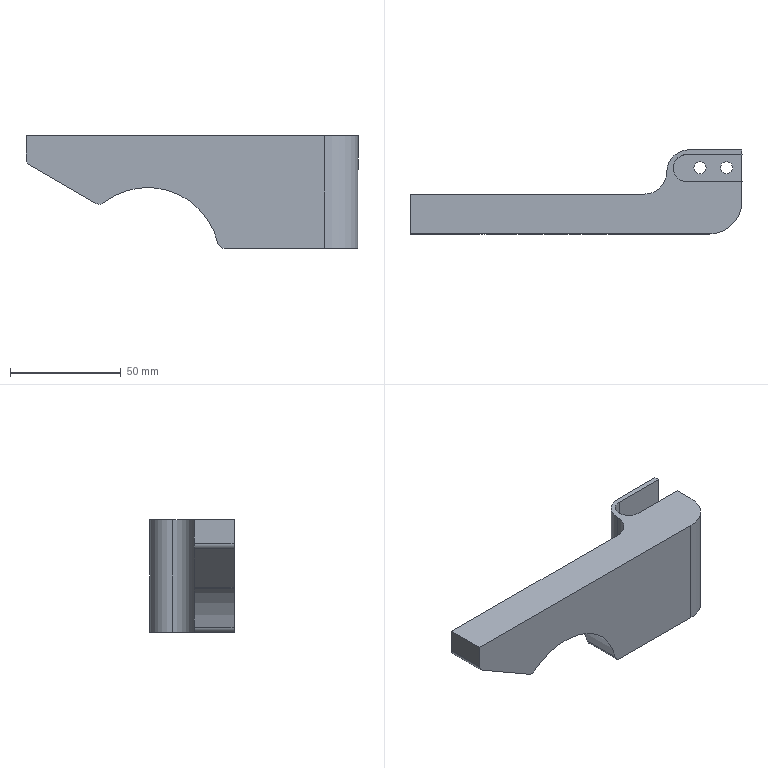NC program | NX | posted with a generic post | part box 150 x 38 x 51 mm
Lines 4811 to 5633 of 31037:
(FIXED_CONTOUR , TOOL : R4)
N9572 T08 M6
N9574 G54
N9576 G17 G0 G90 X11.552 Y21.893 S9500 M3
N9578 G43 Z30. H8
N9580 Z3.895
N9582 G94 G1 X11.585 Y21.86 Z3.374 F3000.
N9584 X11.666 Y21.779 Z2.863
N9586 X11.793 Y21.652 Z2.372
N9588 X11.964 Y21.481 Z1.908
N9590 X12.177 Y21.268 Z1.48
N9592 X12.427 Y21.018 Z1.095
N9594 X12.711 Y20.734 Z0.759
N9596 X13.023 Y20.421 Z0.479
N9598 X13.359 Y20.086 Z0.258
N9600 X13.712 Y19.733 Z0.102
N9602 X14.077 Y19.368 Z0.012
N9604 X14.446 Y18.999 Z-0.01
N9606 X14.583 Y18.862 Z-0.005
N9608 Y18.725 Z-0.004
N9610 X14.309 Y18.999 Z-0.013
N9612 X14.173 Z-0.016
N9614 X14.583 Y18.589 Z-0.003
N9616 Y18.452
N9618 X14.16 Y18.876 Z-0.016
N9620 X14.036 Y19. Z-0.027
N9622 X13.899 Z-0.039
N9624 X14.16 Y18.739 Z-0.014
N9626 X14.583 Y18.316 Z-0.003
N9628 Y18.18
N9630 X14.16 Y18.603 Z-0.013
N9632 X13.877 Y18.886 Z-0.04
N9634 X13.763 Y19. Z-0.054
N9636 X13.626 Z-0.07
N9638 X13.877 Y18.749 Z-0.038
N9640 X14.16 Y18.467 Z-0.013
N9642 X14.583 Y18.043 Z-0.003
N9644 Y17.907
N9646 X14.16 Y18.331 Z-0.013
N9648 X13.84 Y18.65 Z-0.042
N9650 X13.594 Y18.896 Z-0.073
N9652 X13.491 Y19. Z-0.092
N9654 X13.356 Z-0.115
N9656 X13.594 Y18.762 Z-0.071
N9658 X13.877 Y18.479 Z-0.037
N9660 X14.16 Y18.196 Z-0.013
N9662 X14.583 Y17.773 Z-0.003
N9664 Y17.638
N9666 X14.16 Y18.061 Z-0.013
N9668 X13.877 Y18.344 Z-0.037
N9670 X13.594 Y18.626 Z-0.07
N9672 X13.311 Y18.909 Z-0.122
N9674 X13.221 Y19. Z-0.143
N9676 X13.085 Z-0.174
N9678 X13.311 Y18.774 Z-0.121
N9680 X13.594 Y18.491 Z-0.07
N9682 X13.877 Y18.208 Z-0.037
N9684 X14.16 Y17.926 Z-0.013
N9686 X14.583 Y17.502 Z-0.003
N9688 Y17.367
N9690 X14.16 Y17.791 Z-0.013
N9692 X13.877 Y18.073 Z-0.037
N9694 X13.594 Y18.356 Z-0.07
N9696 X13.3 Y18.65 Z-0.122
N9698 X12.95 Y19. Z-0.205
N9700 X12.816 Z-0.236
N9702 X13.165 Y18.65 Z-0.152
N9704 X13.311 Y18.504 Z-0.119
N9706 X13.594 Y18.222 Z-0.07
N9708 X13.877 Y17.939 Z-0.037
N9710 X14.16 Y17.656 Z-0.013
N9712 X14.583 Y17.233 Z-0.003
N9714 Y17.1
N9716 X14.16 Y17.523 Z-0.013
N9718 X13.877 Y17.806 Z-0.037
N9720 X13.594 Y18.088 Z-0.07
N9722 X13.311 Y18.371 Z-0.119
N9724 X13.032 Y18.65 Z-0.182
N9726 X12.746 Y18.937 Z-0.251
N9728 X12.683 Y19. Z-0.27
N9730 X12.549 Z-0.308
N9732 X12.746 Y18.803 Z-0.25
N9734 X13.029 Y18.52 Z-0.183
N9736 X13.311 Y18.237 Z-0.119
N9738 X13.594 Y17.955 Z-0.07
N9740 X13.877 Y17.672 Z-0.037
N9742 X14.16 Y17.389 Z-0.013
N9744 X14.583 Y16.966 Z-0.003
N9746 Y16.832
N9748 X14.16 Y17.256 Z-0.013
N9750 X13.878 Y17.537 Z-0.037
N9752 X13.594 Y17.821 Z-0.07
N9754 X13.311 Y18.104 Z-0.119
N9756 X12.746 Y18.669 Z-0.248
N9758 X12.463 Y18.952 Z-0.332
N9760 X12.415 Y19. Z-0.35
N9762 X12.284 Z-0.398
N9764 X12.463 Y18.821 Z-0.331
N9766 X12.746 Y18.538 Z-0.248
N9768 X13.311 Y17.973 Z-0.119
N9770 X13.594 Y17.69 Z-0.07
N9772 X13.877 Y17.407 Z-0.037
N9774 X14.16 Y17.124 Z-0.013
N9776 X14.583 Y16.701 Z-0.003
N9778 Y16.569
N9780 X14.16 Y16.993 Z-0.013
N9782 X13.877 Y17.275 Z-0.037
N9784 X13.594 Y17.558 Z-0.07
N9786 X13.311 Y17.841 Z-0.119
N9788 X12.746 Y18.406 Z-0.248
N9790 X12.463 Y18.689 Z-0.329
N9792 X12.152 Y19. Z-0.447
N9794 X12.02 Z-0.499
N9796 X12.181 Y18.84 Z-0.434
N9798 X12.463 Y18.557 Z-0.329
N9800 X12.746 Y18.274 Z-0.248
N9802 X13.311 Y17.709 Z-0.119
N9804 X13.594 Y17.426 Z-0.07
N9806 X13.877 Y17.143 Z-0.037
N9808 X14.16 Y16.861 Z-0.013
N9810 X14.583 Y16.437 Z-0.003
N9812 Y16.305
N9814 X14.16 Y16.728 Z-0.013
N9816 X13.877 Y17.011 Z-0.037
N9818 X13.594 Y17.294 Z-0.07
N9820 X13.311 Y17.577 Z-0.119
N9822 X12.746 Y18.142 Z-0.248
N9824 X12.463 Y18.425 Z-0.329
N9826 X12.181 Y18.708 Z-0.433
N9828 X11.888 Y19. Z-0.551
N9830 X11.757 Z-0.605
N9832 X11.898 Y18.859 Z-0.545
N9834 X12.181 Y18.576 Z-0.432
N9836 X12.463 Y18.294 Z-0.329
N9838 X12.746 Y18.011 Z-0.248
N9840 X13.311 Y17.445 Z-0.119
N9842 X13.594 Y17.163 Z-0.07
N9844 X13.877 Y16.88 Z-0.037
N9846 X14.16 Y16.597 Z-0.013
N9848 X14.583 Y16.174 Z-0.003
N9850 Y16.044
N9852 X14.16 Y16.467 Z-0.013
N9854 X13.877 Y16.75 Z-0.037
N9856 X13.594 Y17.032 Z-0.07
N9858 X13.311 Y17.315 Z-0.119
N9860 X12.746 Y17.881 Z-0.248
N9862 X12.463 Y18.163 Z-0.329
N9864 X12.181 Y18.446 Z-0.432
N9866 X11.898 Y18.729 Z-0.544
N9868 X11.626 Y19. Z-0.66
N9870 X11.502 Z-0.722
N9872 X11.615 Y18.887 Z-0.663
N9874 X11.898 Y18.604 Z-0.543
N9876 X12.181 Y18.321 Z-0.432
N9878 X12.463 Y18.039 Z-0.329
N9880 X12.746 Y17.756 Z-0.248
N9882 X13.311 Y17.19 Z-0.119
N9884 X13.594 Y16.908 Z-0.07
N9886 X13.877 Y16.625 Z-0.037
N9888 X14.16 Y16.342 Z-0.013
N9890 X14.583 Y15.919 Z-0.003
N9892 Y15.79
N9894 X14.16 Y16.214 Z-0.013
N9896 X13.877 Y16.496 Z-0.037
N9898 X13.594 Y16.779 Z-0.07
N9900 X13.311 Y17.062 Z-0.119
N9902 X12.746 Y17.627 Z-0.248
N9904 X12.463 Y17.91 Z-0.329
N9906 X12.181 Y18.193 Z-0.432
N9908 X11.898 Y18.475 Z-0.543
N9910 X11.615 Y18.758 Z-0.662
N9912 X11.373 Y19. Z-0.787
N9914 X11.332 Z-0.808
N9916 X11.245 Z-0.858
N9918 X11.332 Y18.913 Z-0.807
N9920 X11.615 Y18.63 Z-0.661
N9922 X11.898 Y18.347 Z-0.543
N9924 X12.181 Y18.065 Z-0.432
N9926 X12.463 Y17.782 Z-0.329
N9928 X12.746 Y17.499 Z-0.248
N9930 X13.311 Y16.934 Z-0.119
N9932 X13.594 Y16.651 Z-0.07
N9934 X13.877 Y16.368 Z-0.037
N9936 X14.16 Y16.085 Z-0.013
N9938 X14.583 Y15.662 Z-0.003
N9940 Y15.536
N9942 X14.16 Y15.959 Z-0.013
N9944 X13.877 Y16.242 Z-0.037
N9946 X13.594 Y16.524 Z-0.07
N9948 X13.311 Y16.807 Z-0.119
N9950 X12.746 Y17.373 Z-0.248
N9952 X12.463 Y17.655 Z-0.329
N9954 X12.181 Y17.938 Z-0.432
N9956 X11.898 Y18.221 Z-0.543
N9958 X11.615 Y18.504 Z-0.661
N9960 X11.332 Y18.786 Z-0.806
N9962 X11.119 Y19. Z-0.931
N9964 X10.994 Z-1.003
N9966 X11.344 Y18.65 Z-0.798
N9968 X11.615 Y18.379 Z-0.661
N9970 X11.902 Y18.092 Z-0.541
N9972 X12.181 Y17.814 Z-0.432
N9974 X12.463 Y17.531 Z-0.329
N9976 X12.746 Y17.248 Z-0.248
N9978 X13.311 Y16.683 Z-0.119
N9980 X13.594 Y16.4 Z-0.07
N9982 X13.877 Y16.117 Z-0.037
N9984 X14.16 Y15.835 Z-0.013
N9986 X14.583 Y15.411 Z-0.003
N9988 Y15.286
N9990 X14.16 Y15.709 Z-0.013
N9992 X13.877 Y15.992 Z-0.037
N9994 X13.594 Y16.275 Z-0.07
N9996 X13.311 Y16.558 Z-0.119
N9998 X12.746 Y17.123 Z-0.248
N10000 X12.463 Y17.406 Z-0.329
N10002 X12.181 Y17.689 Z-0.432
N10004 X11.898 Y17.971 Z-0.543
N10006 X11.615 Y18.254 Z-0.661
N10008 X11.332 Y18.537 Z-0.804
N10010 X11.05 Y18.819 Z-0.969
N10012 X10.869 Y19. Z-1.077
N10014 X10.767 Z-1.137
N10016 X10.743 Z-1.153
N10018 X10.767 Y18.976 Z-1.137
N10020 X11.093 Y18.65 Z-0.942
N10022 X11.332 Y18.411 Z-0.804
N10024 X11.615 Y18.128 Z-0.661
N10026 X11.898 Y17.846 Z-0.543
N10028 X12.181 Y17.563 Z-0.432
N10030 X12.463 Y17.28 Z-0.329
N10032 X12.746 Y16.997 Z-0.248
N10034 X13.311 Y16.432 Z-0.119
N10036 X13.594 Y16.149 Z-0.07
N10038 X13.879 Y15.864 Z-0.037
N10040 X14.16 Y15.584 Z-0.013
N10042 X14.583 Y15.16 Z-0.003
N10044 Y15.039
N10046 X14.16 Y15.462 Z-0.013
N10048 X13.877 Y15.745 Z-0.037
N10050 X13.594 Y16.027 Z-0.07
N10052 X13.311 Y16.31 Z-0.119
N10054 X12.746 Y16.876 Z-0.248
N10056 X12.463 Y17.158 Z-0.329
N10058 X12.181 Y17.441 Z-0.432
N10060 X11.898 Y17.724 Z-0.543
N10062 X11.615 Y18.007 Z-0.661
N10064 X11.332 Y18.289 Z-0.804
N10066 X10.971 Y18.65 Z-1.013
N10068 X10.767 Y18.855 Z-1.135
N10070 X10.622 Y19. Z-1.237
N10072 X10.499 Z-1.322
N10074 X10.767 Y18.733 Z-1.134
N10076 X11.05 Y18.45 Z-0.967
N10078 X11.332 Y18.167 Z-0.804
N10080 X11.615 Y17.884 Z-0.661
N10082 X11.898 Y17.602 Z-0.543
N10084 X12.181 Y17.319 Z-0.432
N10086 X12.463 Y17.036 Z-0.329
N10088 X12.746 Y16.754 Z-0.248
N10090 X13.311 Y16.188 Z-0.119
N10092 X13.594 Y15.905 Z-0.07
N10094 X13.877 Y15.623 Z-0.037
N10096 X14.16 Y15.34 Z-0.013
N10098 X14.583 Y14.917 Z-0.003
N10100 Y14.795
N10102 X14.16 Y15.219 Z-0.013
N10104 X13.877 Y15.501 Z-0.037
N10106 X13.594 Y15.784 Z-0.07
N10108 X13.311 Y16.067 Z-0.119
N10110 X12.746 Y16.632 Z-0.248
N10112 X12.463 Y16.915 Z-0.329
N10114 X12.181 Y17.198 Z-0.432
N10116 X11.898 Y17.481 Z-0.543
N10118 X11.615 Y17.763 Z-0.661
N10120 X11.332 Y18.046 Z-0.804
N10122 X11.05 Y18.329 Z-0.967
N10124 X10.767 Y18.611 Z-1.133
N10126 X10.484 Y18.894 Z-1.331
N10128 X10.378 Y19. Z-1.416
N10130 X10.259 Z-1.511
N10132 X10.484 Y18.775 Z-1.33
N10134 X10.767 Y18.492 Z-1.133
N10136 X11.05 Y18.209 Z-0.967
N10138 X11.332 Y17.926 Z-0.804
N10140 X11.615 Y17.644 Z-0.661
N10142 X11.898 Y17.361 Z-0.543
N10144 X12.181 Y17.078 Z-0.432
N10146 X12.463 Y16.795 Z-0.329
N10148 X12.746 Y16.513 Z-0.248
N10150 X13.311 Y15.947 Z-0.119
N10152 X13.594 Y15.664 Z-0.07
N10154 X13.877 Y15.382 Z-0.037
N10156 X14.16 Y15.099 Z-0.013
N10158 X14.583 Y14.676 Z-0.003
N10160 Y14.558
N10162 X14.16 Y14.982 Z-0.013
N10164 X13.877 Y15.264 Z-0.037
N10166 X13.594 Y15.547 Z-0.07
N10168 X13.311 Y15.83 Z-0.119
N10170 X12.746 Y16.395 Z-0.248
N10172 X12.463 Y16.678 Z-0.329
N10174 X12.181 Y16.961 Z-0.432
N10176 X11.898 Y17.243 Z-0.543
N10178 X11.615 Y17.526 Z-0.661
N10180 X11.332 Y17.809 Z-0.804
N10182 X11.05 Y18.092 Z-0.967
N10184 X10.767 Y18.374 Z-1.133
N10186 X10.484 Y18.657 Z-1.328
N10188 X10.141 Y19. Z-1.605
N10190 X10.027 Z-1.698
N10192 X10.201 Y18.826 Z-1.554
N10194 X10.484 Y18.543 Z-1.328
N10196 X10.767 Y18.26 Z-1.133
N10198 X11.05 Y17.977 Z-0.967
N10200 X11.332 Y17.695 Z-0.804
N10202 X11.615 Y17.412 Z-0.661
N10204 X11.898 Y17.129 Z-0.543
N10206 X12.181 Y16.847 Z-0.432
N10208 X12.463 Y16.564 Z-0.329
N10210 X12.746 Y16.281 Z-0.248
N10212 X13.311 Y15.716 Z-0.119
N10214 X13.594 Y15.433 Z-0.07
N10216 X13.877 Y15.15 Z-0.037
N10218 X14.16 Y14.867 Z-0.013
N10220 X14.583 Y14.444 Z-0.003
N10222 Y14.326
N10224 X14.16 Y14.75 Z-0.013
N10226 X13.877 Y15.033 Z-0.037
N10228 X13.594 Y15.315 Z-0.07
N10230 X13.311 Y15.598 Z-0.119
N10232 X12.746 Y16.163 Z-0.248
N10234 X12.463 Y16.446 Z-0.329
N10236 X12.181 Y16.729 Z-0.432
N10238 X11.898 Y17.012 Z-0.543
N10240 X11.615 Y17.294 Z-0.661
N10242 X11.332 Y17.577 Z-0.804
N10244 X11.05 Y17.86 Z-0.967
N10246 X10.767 Y18.143 Z-1.133
N10248 X10.484 Y18.425 Z-1.328
N10250 X10.201 Y18.708 Z-1.552
N10252 X9.909 Y19. Z-1.795
N10254 X9.798 Z-1.902
N10256 X9.919 Y18.879 Z-1.784
N10258 X10.201 Y18.597 Z-1.551
N10260 X10.484 Y18.314 Z-1.328
N10262 X10.767 Y18.031 Z-1.133
N10264 X11.05 Y17.748 Z-0.967
N10266 X11.332 Y17.466 Z-0.804
N10268 X11.615 Y17.183 Z-0.661
N10270 X11.898 Y16.9 Z-0.543
N10272 X12.181 Y16.617 Z-0.432
N10274 X12.463 Y16.335 Z-0.329
N10276 X12.746 Y16.052 Z-0.248
N10278 X13.311 Y15.486 Z-0.119
N10280 X13.594 Y15.204 Z-0.07
N10282 X13.877 Y14.921 Z-0.037
N10284 X14.16 Y14.638 Z-0.013
N10286 X14.583 Y14.215 Z-0.003
N10288 Y14.102
N10290 X14.16 Y14.525 Z-0.013
N10292 X13.877 Y14.808 Z-0.037
N10294 X13.594 Y15.091 Z-0.07
N10296 X13.311 Y15.374 Z-0.119
N10298 X12.746 Y15.939 Z-0.248
N10300 X12.463 Y16.222 Z-0.329
N10302 X12.181 Y16.505 Z-0.432
N10304 X11.898 Y16.787 Z-0.543
N10306 X11.615 Y17.07 Z-0.661
N10308 X11.332 Y17.353 Z-0.804
N10310 X11.05 Y17.636 Z-0.967
N10312 X10.767 Y17.918 Z-1.133
N10314 X10.484 Y18.201 Z-1.328
N10316 X10.201 Y18.484 Z-1.551
N10318 X9.919 Y18.766 Z-1.783
N10320 X9.685 Y19. Z-2.01
N10322 X9.636 Z-2.056
N10324 X9.572 Z-2.124
N10326 X9.636 Y18.936 Z-2.054
N10328 X9.919 Y18.654 Z-1.781
N10330 X10.201 Y18.371 Z-1.551
N10332 X10.484 Y18.088 Z-1.328
N10334 X10.767 Y17.806 Z-1.133
N10336 X11.05 Y17.523 Z-0.967
N10338 X11.332 Y17.24 Z-0.804
N10340 X11.615 Y16.957 Z-0.661
N10342 X11.898 Y16.675 Z-0.543
N10344 X12.181 Y16.392 Z-0.432
N10346 X12.463 Y16.109 Z-0.329
N10348 X12.746 Y15.826 Z-0.248
N10350 X13.311 Y15.261 Z-0.119
N10352 X13.594 Y14.978 Z-0.07
N10354 X13.877 Y14.695 Z-0.037
N10356 X14.16 Y14.413 Z-0.013
N10358 X14.583 Y13.989 Z-0.003
N10360 Y13.88
N10362 X14.16 Y14.303 Z-0.013
N10364 X13.877 Y14.586 Z-0.037
N10366 X13.594 Y14.869 Z-0.07
N10368 X13.311 Y15.151 Z-0.119
N10370 X12.746 Y15.717 Z-0.248
N10372 X12.463 Y16. Z-0.329
N10374 X12.181 Y16.282 Z-0.432
N10376 X11.898 Y16.565 Z-0.543
N10378 X11.615 Y16.848 Z-0.661
N10380 X11.332 Y17.131 Z-0.804
N10382 X11.05 Y17.413 Z-0.967
N10384 X10.767 Y17.696 Z-1.133
N10386 X10.484 Y17.979 Z-1.328
N10388 X10.201 Y18.262 Z-1.551
N10390 X9.919 Y18.544 Z-1.781
N10392 X9.636 Y18.827 Z-2.053
N10394 X9.463 Y19. Z-2.241
N10396 X9.357 Z-2.355
N10398 X9.636 Y18.721 Z-2.053
N10400 X9.919 Y18.438 Z-1.781
N10402 X10.201 Y18.156 Z-1.551
N10404 X10.484 Y17.873 Z-1.328
N10406 X10.767 Y17.59 Z-1.133
N10408 X11.05 Y17.307 Z-0.967
N10410 X11.332 Y17.025 Z-0.804
N10412 X11.615 Y16.742 Z-0.661
N10414 X11.898 Y16.459 Z-0.543
N10416 X12.181 Y16.176 Z-0.432
N10418 X12.463 Y15.894 Z-0.329
N10420 X12.746 Y15.611 Z-0.248
N10422 X13.311 Y15.045 Z-0.119
N10424 X13.594 Y14.763 Z-0.07
N10426 X13.877 Y14.48 Z-0.037
N10428 X14.16 Y14.197 Z-0.013
N10430 X14.583 Y13.774 Z-0.003
N10432 Y13.669
N10434 X14.16 Y14.092 Z-0.013
N10436 X13.877 Y14.375 Z-0.037
N10438 X13.594 Y14.657 Z-0.07
N10440 X13.311 Y14.94 Z-0.119
N10442 X12.746 Y15.506 Z-0.248
N10444 X12.463 Y15.788 Z-0.329
N10446 X12.181 Y16.071 Z-0.432
N10448 X11.898 Y16.354 Z-0.543
N10450 X11.615 Y16.637 Z-0.661
N10452 X11.332 Y16.919 Z-0.804
N10454 X11.05 Y17.202 Z-0.967
N10456 X10.767 Y17.485 Z-1.133
N10458 X10.484 Y17.768 Z-1.328
N10460 X10.201 Y18.05 Z-1.551
N10462 X9.919 Y18.333 Z-1.781
N10464 X9.636 Y18.616 Z-2.053
N10466 X9.353 Y18.898 Z-2.357
N10468 X9.252 Y19. Z-2.477
N10470 X9.147 Z-2.599
N10472 X9.353 Y18.794 Z-2.357
N10474 X9.636 Y18.511 Z-2.053
N10476 X9.919 Y18.229 Z-1.781
N10478 X10.201 Y17.946 Z-1.551
N10480 X10.484 Y17.663 Z-1.328
N10482 X10.767 Y17.381 Z-1.133
N10484 X11.05 Y17.098 Z-0.967
N10486 X11.332 Y16.815 Z-0.804
N10488 X11.615 Y16.532 Z-0.661
N10490 X11.898 Y16.25 Z-0.543
N10492 X12.181 Y15.967 Z-0.432
N10494 X12.463 Y15.684 Z-0.329
N10496 X12.746 Y15.401 Z-0.248
N10498 X13.311 Y14.836 Z-0.119
N10500 X13.594 Y14.553 Z-0.07
N10502 X13.877 Y14.27 Z-0.037
N10504 X14.16 Y13.988 Z-0.013
N10506 X14.583 Y13.564 Z-0.003
N10508 Y13.464
N10510 X14.16 Y13.887 Z-0.013
N10512 X13.877 Y14.17 Z-0.037
N10514 X13.594 Y14.453 Z-0.07
N10516 X13.311 Y14.736 Z-0.119
N10518 X12.746 Y15.301 Z-0.248
N10520 X12.463 Y15.584 Z-0.329
N10522 X12.183 Y15.864 Z-0.431
N10524 X11.898 Y16.149 Z-0.543
N10526 X11.615 Y16.432 Z-0.661
N10528 X11.332 Y16.715 Z-0.804
N10530 X11.057 Y16.99 Z-0.963
N10532 X10.767 Y17.28 Z-1.133
N10534 X10.484 Y17.563 Z-1.328
N10536 X10.201 Y17.846 Z-1.551
N10538 X9.919 Y18.128 Z-1.781
N10540 X9.636 Y18.411 Z-2.053
N10542 X9.353 Y18.694 Z-2.357
N10544 X9.07 Y18.977 Z-2.687
N10546 X9.047 Y19. Z-2.722
N10548 X8.951 Z-2.858
N10550 X9.07 Y18.881 Z-2.686
N10552 X9.353 Y18.598 Z-2.357
N10554 X9.636 Y18.315 Z-2.053
N10556 X9.919 Y18.033 Z-1.781
N10558 X10.201 Y17.75 Z-1.551
N10560 X10.484 Y17.467 Z-1.328
N10562 X10.767 Y17.184 Z-1.133
N10564 X11.05 Y16.902 Z-0.967
N10566 X11.332 Y16.619 Z-0.804
N10568 X11.615 Y16.336 Z-0.661
N10570 X11.898 Y16.053 Z-0.543
N10572 X12.181 Y15.771 Z-0.432
N10574 X12.463 Y15.488 Z-0.329
N10576 X12.746 Y15.205 Z-0.248
N10578 X13.311 Y14.64 Z-0.119
N10580 X13.594 Y14.357 Z-0.07
N10582 X13.877 Y14.074 Z-0.037
N10584 X14.16 Y13.792 Z-0.013
N10586 X14.583 Y13.368 Z-0.003
N10588 Y13.271
N10590 X14.16 Y13.695 Z-0.013
N10592 X13.877 Y13.977 Z-0.037
N10594 X13.594 Y14.26 Z-0.07
N10596 X13.311 Y14.543 Z-0.119
N10598 X12.746 Y15.108 Z-0.248
N10600 X12.463 Y15.391 Z-0.329
N10602 X12.181 Y15.674 Z-0.432
N10604 X11.898 Y15.956 Z-0.543
N10606 X11.615 Y16.239 Z-0.661
N10608 X11.332 Y16.522 Z-0.804
N10610 X11.05 Y16.805 Z-0.967
N10612 X10.767 Y17.087 Z-1.133
N10614 X10.484 Y17.37 Z-1.328
N10616 X10.201 Y17.653 Z-1.551
N10618 X9.919 Y17.936 Z-1.781
N10620 X9.636 Y18.218 Z-2.053
N10622 X9.353 Y18.501 Z-2.357
N10624 X9.07 Y18.784 Z-2.686
N10626 X8.854 Y19. Z-2.996
N10628 X8.788 Z-3.091
N10630 X8.758 Z-3.137
N10632 X8.788 Y18.97 Z-3.09
N10634 X9.07 Y18.687 Z-2.686
N10636 X9.353 Y18.405 Z-2.357
N10638 X9.636 Y18.122 Z-2.053
N10640 X9.919 Y17.839 Z-1.781
N10642 X10.201 Y17.556 Z-1.551
N10644 X10.484 Y17.274 Z-1.328
N10646 X10.767 Y16.991 Z-1.133
N10648 X11.05 Y16.708 Z-0.967
N10650 X11.332 Y16.426 Z-0.804
N10652 X11.615 Y16.143 Z-0.661
N10654 X11.898 Y15.86 Z-0.543
N10656 X12.181 Y15.577 Z-0.432
N10658 X12.463 Y15.295 Z-0.329
N10660 X12.746 Y15.012 Z-0.248
N10662 X13.311 Y14.446 Z-0.119
N10664 X13.594 Y14.164 Z-0.07
N10666 X13.877 Y13.881 Z-0.037
N10668 X14.16 Y13.598 Z-0.013
N10670 X14.583 Y13.175 Z-0.003
N10672 Y13.083
N10674 X14.16 Y13.506 Z-0.013
N10676 X13.877 Y13.789 Z-0.037
N10678 X13.594 Y14.072 Z-0.07
N10680 X13.311 Y14.355 Z-0.119
N10682 X12.746 Y14.92 Z-0.248
N10684 X12.463 Y15.203 Z-0.329
N10686 X12.181 Y15.485 Z-0.432
N10688 X11.898 Y15.768 Z-0.543
N10690 X11.615 Y16.051 Z-0.661
N10692 X11.332 Y16.334 Z-0.804
N10694 X11.05 Y16.616 Z-0.967
N10696 X10.767 Y16.899 Z-1.133
N10698 X10.484 Y17.182 Z-1.328
N10700 X10.201 Y17.465 Z-1.551
N10702 X9.919 Y17.747 Z-1.781
N10704 X9.636 Y18.03 Z-2.053
N10706 X9.353 Y18.313 Z-2.357
N10708 X9.07 Y18.596 Z-2.686
N10710 X8.788 Y18.878 Z-3.088
N10712 X8.666 Y19. Z-3.28
N10714 X8.573 Z-3.424
N10716 X8.788 Y18.786 Z-3.088
N10718 X9.07 Y18.503 Z-2.686
N10720 X9.353 Y18.22 Z-2.357
N10722 X9.636 Y17.938 Z-2.053
N10724 X9.919 Y17.655 Z-1.781
N10726 X10.201 Y17.372 Z-1.551
N10728 X10.484 Y17.089 Z-1.328
N10730 X10.767 Y16.807 Z-1.133
N10732 X11.05 Y16.524 Z-0.967
N10734 X11.332 Y16.241 Z-0.804
N10736 X11.615 Y15.958 Z-0.661
N10738 X11.898 Y15.676 Z-0.543
N10740 X12.181 Y15.393 Z-0.432
N10742 X12.463 Y15.11 Z-0.329
N10744 X12.746 Y14.827 Z-0.248
N10746 X13.311 Y14.262 Z-0.119
N10748 X13.594 Y13.979 Z-0.07
N10750 X13.877 Y13.697 Z-0.037
N10752 X14.16 Y13.414 Z-0.013
N10754 X14.583 Y12.99 Z-0.003
N10756 Y12.9
N10758 X14.16 Y13.323 Z-0.013
N10760 X13.877 Y13.606 Z-0.037
N10762 X13.594 Y13.889 Z-0.07
N10764 X13.311 Y14.171 Z-0.119
N10766 X12.746 Y14.737 Z-0.248
N10768 X12.463 Y15.02 Z-0.329
N10770 X12.181 Y15.302 Z-0.432
N10772 X11.898 Y15.585 Z-0.543
N10774 X11.615 Y15.868 Z-0.661
N10776 X11.332 Y16.151 Z-0.804
N10778 X11.055 Y16.428 Z-0.964
N10780 X10.767 Y16.716 Z-1.133
N10782 X10.484 Y16.999 Z-1.328
N10784 X10.201 Y17.281 Z-1.551
N10786 X9.919 Y17.564 Z-1.781
N10788 X9.636 Y17.847 Z-2.053
N10790 X9.353 Y18.13 Z-2.357
N10792 X9.07 Y18.412 Z-2.686
N10794 X8.788 Y18.695 Z-3.088
N10796 X8.505 Y18.978 Z-3.529
N10798 X8.483 Y19. Z-3.573
N10800 X8.406 Z-3.725
N10802 X8.505 Y18.901 Z-3.528
N10804 X8.788 Y18.618 Z-3.088
N10806 X9.07 Y18.336 Z-2.686
N10808 X9.353 Y18.053 Z-2.357
N10810 X9.636 Y17.77 Z-2.053
N10812 X9.919 Y17.487 Z-1.781
N10814 X10.201 Y17.205 Z-1.551
N10816 X10.484 Y16.922 Z-1.328
N10818 X10.767 Y16.639 Z-1.133
N10820 X11.05 Y16.356 Z-0.967
N10822 X11.332 Y16.074 Z-0.804
N10824 X11.615 Y15.791 Z-0.661
N10826 X11.898 Y15.508 Z-0.543
N10828 X12.181 Y15.226 Z-0.432
N10830 X12.463 Y14.943 Z-0.329
N10832 X12.746 Y14.66 Z-0.248
N10834 X13.311 Y14.095 Z-0.119
N10836 X13.594 Y13.812 Z-0.07
N10838 X13.877 Y13.529 Z-0.037
N10840 X14.16 Y13.246 Z-0.013
N10842 X14.583 Y12.823 Z-0.003
N10844 Y12.742
N10846 X14.16 Y13.165 Z-0.013
N10848 X13.877 Y13.448 Z-0.037
N10850 X13.594 Y13.73 Z-0.07
N10852 X13.311 Y14.013 Z-0.119
N10854 X12.746 Y14.579 Z-0.248
N10856 X12.463 Y14.861 Z-0.329
N10858 X12.181 Y15.144 Z-0.432
N10860 X11.898 Y15.427 Z-0.543
N10862 X11.615 Y15.71 Z-0.661
N10864 X11.332 Y15.992 Z-0.804
N10866 X11.05 Y16.275 Z-0.967
N10868 X10.767 Y16.558 Z-1.133
N10870 X10.484 Y16.84 Z-1.328
N10872 X10.201 Y17.123 Z-1.551
N10874 X9.919 Y17.406 Z-1.781
N10876 X9.636 Y17.689 Z-2.053
N10878 X9.353 Y17.971 Z-2.357
N10880 X9.07 Y18.254 Z-2.686
N10882 X8.788 Y18.537 Z-3.088
N10884 X8.505 Y18.82 Z-3.528
N10886 X8.364 Y18.961 Z-3.808
N10888 X8.325 Y19. Z-3.89
N10890 X8.242 Z-4.06
N10892 X8.364 Y18.878 Z-3.806
N10894 X8.437 Y18.805 Z-3.659
N10896 X8.505 Y18.737 Z-3.528
N10898 X8.788 Y18.454 Z-3.088
N10900 X9.07 Y18.172 Z-2.686
N10902 X9.353 Y17.889 Z-2.357
N10904 X9.636 Y17.606 Z-2.053
N10906 X9.919 Y17.323 Z-1.781
N10908 X10.201 Y17.041 Z-1.551
N10910 X10.484 Y16.758 Z-1.328
N10912 X10.767 Y16.475 Z-1.133
N10914 X11.05 Y16.192 Z-0.967
N10916 X11.332 Y15.91 Z-0.804
N10918 X11.615 Y15.627 Z-0.661
N10920 X11.898 Y15.344 Z-0.543
N10922 X12.181 Y15.062 Z-0.432
N10924 X12.463 Y14.779 Z-0.329
N10926 X12.746 Y14.496 Z-0.248
N10928 X13.311 Y13.931 Z-0.119
N10930 X13.594 Y13.648 Z-0.07
N10932 X13.877 Y13.365 Z-0.037
N10934 X14.16 Y13.082 Z-0.013
N10936 X14.583 Y12.659 Z-0.003
N10938 Y12.579
N10940 X14.16 Y13.003 Z-0.013
N10942 X13.877 Y13.285 Z-0.037
N10944 X13.594 Y13.568 Z-0.07
N10946 X13.311 Y13.851 Z-0.119
N10948 X12.746 Y14.416 Z-0.248
N10950 X12.463 Y14.699 Z-0.329
N10952 X12.181 Y14.982 Z-0.432
N10954 X11.898 Y15.265 Z-0.543
N10956 X11.615 Y15.547 Z-0.661
N10958 X11.332 Y15.83 Z-0.804
N10960 X11.05 Y16.113 Z-0.967
N10962 X10.767 Y16.395 Z-1.133
N10964 X10.484 Y16.678 Z-1.328
N10966 X10.201 Y16.961 Z-1.551
N10968 X9.919 Y17.244 Z-1.781
N10970 X9.636 Y17.526 Z-2.053
N10972 X9.353 Y17.809 Z-2.357
N10974 X9.071 Y18.091 Z-2.686
N10976 X8.788 Y18.375 Z-3.088
N10978 X8.505 Y18.657 Z-3.528
N10980 X8.412 Y18.751 Z-3.708
N10982 X8.364 Y18.799 Z-3.805
N10984 X8.222 Y18.94 Z-4.1
N10986 X8.162 Y19. Z-4.235
N10988 X8.086 Z-4.404
N10990 X8.222 Y18.864 Z-4.098
N10992 X8.387 Y18.699 Z-3.756
N10994 X8.505 Y18.581 Z-3.528
N10996 X8.788 Y18.299 Z-3.088
N10998 X9.07 Y18.016 Z-2.686
N11000 X9.353 Y17.733 Z-2.357
N11002 X9.636 Y17.45 Z-2.053
N11004 X9.919 Y17.168 Z-1.781
N11006 X10.201 Y16.885 Z-1.551
N11008 X10.484 Y16.602 Z-1.328
N11010 X10.767 Y16.319 Z-1.133
N11012 X11.05 Y16.037 Z-0.967
N11014 X11.332 Y15.754 Z-0.804
N11016 X11.615 Y15.471 Z-0.661
N11018 X11.898 Y15.189 Z-0.543
N11020 X12.181 Y14.906 Z-0.432
N11022 X12.463 Y14.623 Z-0.329
N11024 X12.746 Y14.34 Z-0.248
N11026 X13.311 Y13.775 Z-0.119
N11028 X13.594 Y13.492 Z-0.07
N11030 X13.877 Y13.209 Z-0.037
N11032 X14.16 Y12.927 Z-0.013
N11034 X14.583 Y12.503 Z-0.003
N11036 Y12.444
N11038 X14.16 Y12.868 Z-0.013
N11040 X13.877 Y13.15 Z-0.037
N11042 X13.594 Y13.433 Z-0.07
N11044 X13.311 Y13.716 Z-0.119
N11046 X12.746 Y14.281 Z-0.248
N11048 X12.463 Y14.564 Z-0.329
N11050 X12.181 Y14.847 Z-0.432
N11052 X11.898 Y15.129 Z-0.543
N11054 X11.615 Y15.412 Z-0.661
N11056 X11.332 Y15.695 Z-0.804
N11058 X11.05 Y15.978 Z-0.967
N11060 X10.767 Y16.26 Z-1.133
N11062 X10.484 Y16.543 Z-1.328
N11064 X10.201 Y16.826 Z-1.551
N11066 X9.919 Y17.108 Z-1.781
N11068 X9.636 Y17.391 Z-2.053
N11070 X9.353 Y17.674 Z-2.357
N11072 X9.07 Y17.957 Z-2.686
N11074 X8.788 Y18.239 Z-3.088
N11076 X8.505 Y18.522 Z-3.528
N11078 X8.364 Y18.664 Z-3.802
N11080 X8.222 Y18.805 Z-4.097
N11082 X8.081 Y18.946 Z-4.415
N11084 X8.027 Y19. Z-4.569
N11086 X7.963 Z-4.752
N11088 X8.081 Y18.882 Z-4.413
N11090 X8.222 Y18.74 Z-4.095
N11092 X8.364 Y18.599 Z-3.801
N11094 X8.505 Y18.458 Z-3.528
N11096 X8.788 Y18.175 Z-3.088
N11098 X9.07 Y17.892 Z-2.686
N11100 X9.353 Y17.61 Z-2.357
N11102 X9.636 Y17.327 Z-2.053
N11104 X9.919 Y17.044 Z-1.781
N11106 X10.201 Y16.761 Z-1.551
N11108 X10.484 Y16.479 Z-1.328
N11110 X10.767 Y16.196 Z-1.133
N11112 X11.05 Y15.913 Z-0.967
N11114 X11.332 Y15.63 Z-0.804
N11116 X11.615 Y15.348 Z-0.661
N11118 X11.898 Y15.065 Z-0.543
N11120 X12.181 Y14.782 Z-0.432
N11122 X12.463 Y14.499 Z-0.329
N11124 X12.746 Y14.217 Z-0.248
N11126 X13.311 Y13.651 Z-0.119
N11128 X13.594 Y13.369 Z-0.07
N11130 X13.877 Y13.086 Z-0.037
N11132 X14.16 Y12.803 Z-0.013
N11134 X14.583 Y12.38 Z-0.003
N11136 Y12.318
N11138 X14.16 Y12.741 Z-0.013
N11140 X13.877 Y13.024 Z-0.037
N11142 X13.594 Y13.307 Z-0.07
N11144 X13.311 Y13.59 Z-0.119
N11146 X12.746 Y14.155 Z-0.248
N11148 X12.463 Y14.438 Z-0.329
N11150 X12.181 Y14.721 Z-0.432
N11152 X11.898 Y15.003 Z-0.543
N11154 X11.615 Y15.286 Z-0.661
N11156 X11.332 Y15.569 Z-0.804
N11158 X11.05 Y15.851 Z-0.967
N11160 X10.767 Y16.134 Z-1.133
N11162 X10.484 Y16.417 Z-1.328
N11164 X10.201 Y16.7 Z-1.551
N11166 X9.919 Y16.982 Z-1.781
N11168 X9.636 Y17.265 Z-2.053
N11170 X9.353 Y17.548 Z-2.357
N11172 X9.07 Y17.831 Z-2.686
N11174 X8.788 Y18.113 Z-3.088
N11176 X8.505 Y18.396 Z-3.528
N11178 X8.364 Y18.537 Z-3.801
N11180 X8.222 Y18.679 Z-4.094
N11182 X8.081 Y18.82 Z-4.411
N11184 X7.94 Y18.961 Z-4.819
N11186 X7.901 Y19. Z-4.948
N11188 X7.845 Z-5.136
N11190 X7.94 Y18.906 Z-4.818
N11192 X8.081 Y18.765 Z-4.41
N11194 X8.222 Y18.623 Z-4.093
N11196 X8.364 Y18.482 Z-3.801
N11198 X8.505 Y18.34 Z-3.528
N11200 X8.788 Y18.058 Z-3.088
N11202 X9.07 Y17.775 Z-2.686
N11204 X9.353 Y17.492 Z-2.357
N11206 X9.636 Y17.209 Z-2.053
N11208 X9.919 Y16.927 Z-1.781
N11210 X10.201 Y16.644 Z-1.551